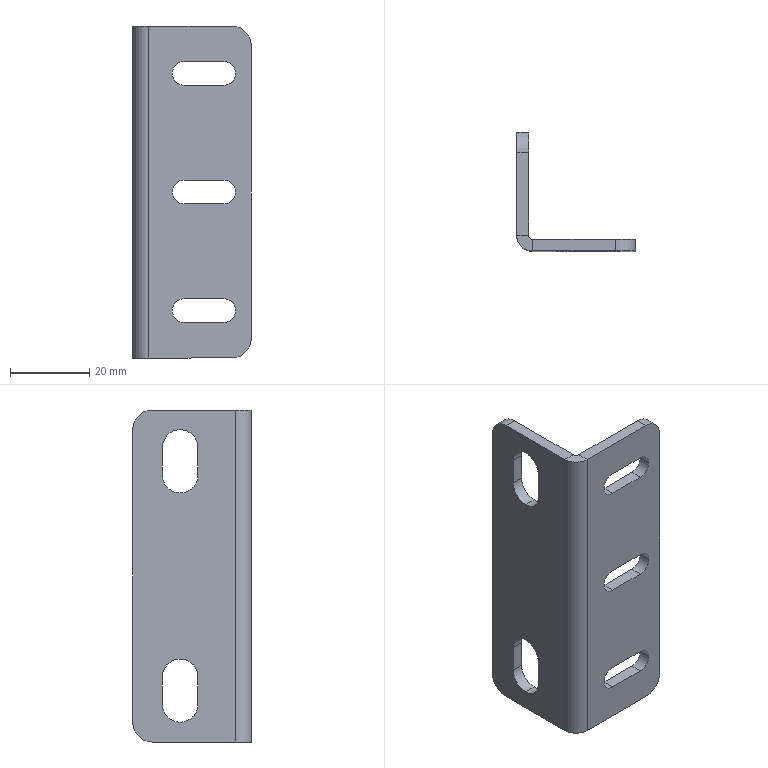Part | SolidWorks | features HoleWzd 2, EdgeFlange 1, Fillet 1, FlatPattern 1, SMBaseFlange 1, SheetMetal 1 | 1 solid | 40 faces | box 30 x 30 x 84 mm | volume 12475 mm3 | plane 22 | cylinder 18 | commonest cylinder face diameters 6 x6 9 x6 10 x4 2 x1 8 x1
STEP:
#1=CARTESIAN_POINT('',(-15.,15.,-37.));
#2=VERTEX_POINT('',#1);
#3=CARTESIAN_POINT('',(-15.,19.5,-32.5));
#4=VERTEX_POINT('',#3);
#5=CARTESIAN_POINT('',(-15.,15.,-32.5));
#6=DIRECTION('',(1.,0.,0.));
#7=DIRECTION('',(0.,0.,-1.));
#8=AXIS2_PLACEMENT_3D('',#5,#6,#7);
#9=CIRCLE('',#8,4.5);
#10=EDGE_CURVE('',#2,#4,#9,.T.);
#11=ORIENTED_EDGE('',*,*,#10,.F.);
#12=CARTESIAN_POINT('',(-12.,15.,-37.));
#13=VERTEX_POINT('',#12);
#14=CARTESIAN_POINT('',(-12.,15.,-37.));
#15=DIRECTION('',(1.,0.,0.));
#16=VECTOR('',#15,1000.);
#17=LINE('',#14,#16);
#18=EDGE_CURVE('',#2,#13,#17,.T.);
#19=ORIENTED_EDGE('',*,*,#18,.T.);
#20=CARTESIAN_POINT('',(-12.,19.5,-32.5));
#21=VERTEX_POINT('',#20);
#22=CARTESIAN_POINT('',(-12.,15.,-32.5));
#23=DIRECTION('',(1.,0.,0.));
#24=DIRECTION('',(0.,0.,-1.));
#25=AXIS2_PLACEMENT_3D('',#22,#23,#24);
#26=CIRCLE('',#25,4.5);
#27=EDGE_CURVE('',#13,#21,#26,.T.);
#28=ORIENTED_EDGE('',*,*,#27,.T.);
#29=CARTESIAN_POINT('',(-15.,19.5,-32.5));
#30=DIRECTION('',(-1.,0.,0.));
#31=VECTOR('',#30,1000.);
#32=LINE('',#29,#31);
#33=EDGE_CURVE('',#21,#4,#32,.T.);
#34=ORIENTED_EDGE('',*,*,#33,.T.);
#35=EDGE_LOOP('',(#11,#19,#28,#34));
#36=FACE_OUTER_BOUND('',#35,.T.);
#37=CARTESIAN_POINT('',(-12.,15.,-32.5));
#38=DIRECTION('',(1.,0.,0.));
#39=DIRECTION('',(0.,0.,-1.));
#40=AXIS2_PLACEMENT_3D('',#37,#38,#39);
#41=CYLINDRICAL_SURFACE('',#40,4.5);
#42=ADVANCED_FACE('',(#36),#41,.F.);
#43=CARTESIAN_POINT('',(-15.,15.,21.));
#44=VERTEX_POINT('',#43);
#45=CARTESIAN_POINT('',(-15.,19.5,25.5));
#46=VERTEX_POINT('',#45);
#47=CARTESIAN_POINT('',(-15.,15.,25.5));
#48=DIRECTION('',(1.,0.,0.));
#49=DIRECTION('',(0.,0.,-1.));
#50=AXIS2_PLACEMENT_3D('',#47,#48,#49);
#51=CIRCLE('',#50,4.5);
#52=EDGE_CURVE('',#44,#46,#51,.T.);
#53=ORIENTED_EDGE('',*,*,#52,.F.);
#54=CARTESIAN_POINT('',(-12.,15.,21.));
#55=VERTEX_POINT('',#54);
#56=CARTESIAN_POINT('',(-12.,15.,21.));
#57=DIRECTION('',(1.,0.,0.));
#58=VECTOR('',#57,1000.);
#59=LINE('',#56,#58);
#60=EDGE_CURVE('',#44,#55,#59,.T.);
#61=ORIENTED_EDGE('',*,*,#60,.T.);
#62=CARTESIAN_POINT('',(-12.,19.5,25.5));
#63=VERTEX_POINT('',#62);
#64=CARTESIAN_POINT('',(-12.,15.,25.5));
#65=DIRECTION('',(1.,0.,0.));
#66=DIRECTION('',(0.,0.,-1.));
#67=AXIS2_PLACEMENT_3D('',#64,#65,#66);
#68=CIRCLE('',#67,4.5);
#69=EDGE_CURVE('',#55,#63,#68,.T.);
#70=ORIENTED_EDGE('',*,*,#69,.T.);
#71=CARTESIAN_POINT('',(-15.,19.5,25.5));
#72=DIRECTION('',(-1.,0.,0.));
#73=VECTOR('',#72,1000.);
#74=LINE('',#71,#73);
#75=EDGE_CURVE('',#63,#46,#74,.T.);
#76=ORIENTED_EDGE('',*,*,#75,.T.);
#77=EDGE_LOOP('',(#53,#61,#70,#76));
#78=FACE_OUTER_BOUND('',#77,.T.);
#79=CARTESIAN_POINT('',(-12.,15.,25.5));
#80=DIRECTION('',(1.,0.,0.));
#81=DIRECTION('',(0.,0.,-1.));
#82=AXIS2_PLACEMENT_3D('',#79,#80,#81);
#83=CYLINDRICAL_SURFACE('',#82,4.5);
#84=ADVANCED_FACE('',(#78),#83,.F.);
#85=CARTESIAN_POINT('',(-15.,10.5,-32.5));
#86=VERTEX_POINT('',#85);
#87=CARTESIAN_POINT('',(-15.,15.,-32.5));
#88=DIRECTION('',(1.,0.,0.));
#89=DIRECTION('',(0.,0.,-1.));
#90=AXIS2_PLACEMENT_3D('',#87,#88,#89);
#91=CIRCLE('',#90,4.5);
#92=EDGE_CURVE('',#86,#2,#91,.T.);
#93=ORIENTED_EDGE('',*,*,#92,.T.);
#94=ORIENTED_EDGE('',*,*,#10,.T.);
#95=CARTESIAN_POINT('',(-15.,19.5,-25.5));
#96=VERTEX_POINT('',#95);
#97=CARTESIAN_POINT('',(-15.,19.5,-32.5));
#98=DIRECTION('',(0.,0.,1.));
#99=VECTOR('',#98,1000.);
#100=LINE('',#97,#99);
#101=EDGE_CURVE('',#4,#96,#100,.T.);
#102=ORIENTED_EDGE('',*,*,#101,.T.);
#103=CARTESIAN_POINT('',(-15.,10.5,-25.5));
#104=VERTEX_POINT('',#103);
#105=CARTESIAN_POINT('',(-15.,15.,-25.5));
#106=DIRECTION('',(1.,0.,0.));
#107=DIRECTION('',(0.,0.,-1.));
#108=AXIS2_PLACEMENT_3D('',#105,#106,#107);
#109=CIRCLE('',#108,4.5);
#110=EDGE_CURVE('',#96,#104,#109,.T.);
#111=ORIENTED_EDGE('',*,*,#110,.T.);
#112=CARTESIAN_POINT('',(-15.,10.5,-32.5));
#113=DIRECTION('',(0.,0.,1.));
#114=VECTOR('',#113,1000.);
#115=LINE('',#112,#114);
#116=EDGE_CURVE('',#86,#104,#115,.T.);
#117=ORIENTED_EDGE('',*,*,#116,.F.);
#118=EDGE_LOOP('',(#93,#94,#102,#111,#117));
#119=FACE_BOUND('',#118,.T.);
#120=CARTESIAN_POINT('',(-15.,27.,37.));
#121=VERTEX_POINT('',#120);
#122=CARTESIAN_POINT('',(-15.,27.,-37.));
#123=VERTEX_POINT('',#122);
#124=CARTESIAN_POINT('',(-15.,27.,0.));
#125=DIRECTION('',(0.,0.,-1.));
#126=VECTOR('',#125,1000.);
#127=LINE('',#124,#126);
#128=EDGE_CURVE('',#121,#123,#127,.T.);
#129=ORIENTED_EDGE('',*,*,#128,.T.);
#130=CARTESIAN_POINT('',(-15.,22.,-42.));
#131=VERTEX_POINT('',#130);
#132=CARTESIAN_POINT('',(-15.,22.,-37.));
#133=DIRECTION('',(-1.,0.,0.));
#134=DIRECTION('',(0.,1.,0.));
#135=AXIS2_PLACEMENT_3D('',#132,#133,#134);
#136=CIRCLE('',#135,5.);
#137=EDGE_CURVE('',#123,#131,#136,.T.);
#138=ORIENTED_EDGE('',*,*,#137,.T.);
#139=CARTESIAN_POINT('',(-15.,1.,-42.));
#140=VERTEX_POINT('',#139);
#141=CARTESIAN_POINT('',(-15.,0.,-42.));
#142=DIRECTION('',(0.,-1.,0.));
#143=VECTOR('',#142,1000.);
#144=LINE('',#141,#143);
#145=EDGE_CURVE('',#131,#140,#144,.T.);
#146=ORIENTED_EDGE('',*,*,#145,.T.);
#147=CARTESIAN_POINT('',(-15.,1.,42.));
#148=VERTEX_POINT('',#147);
#149=CARTESIAN_POINT('',(-15.,1.,-42.));
#150=DIRECTION('',(0.,0.,-1.));
#151=VECTOR('',#150,1000.);
#152=LINE('',#149,#151);
#153=EDGE_CURVE('',#148,#140,#152,.T.);
#154=ORIENTED_EDGE('',*,*,#153,.F.);
#155=CARTESIAN_POINT('',(-15.,22.,42.));
#156=VERTEX_POINT('',#155);
#157=CARTESIAN_POINT('',(-15.,0.,42.));
#158=DIRECTION('',(0.,1.,0.));
#159=VECTOR('',#158,1000.);
#160=LINE('',#157,#159);
#161=EDGE_CURVE('',#148,#156,#160,.T.);
#162=ORIENTED_EDGE('',*,*,#161,.T.);
#163=CARTESIAN_POINT('',(-15.,22.,37.));
#164=DIRECTION('',(-1.,0.,0.));
#165=DIRECTION('',(0.,1.,0.));
#166=AXIS2_PLACEMENT_3D('',#163,#164,#165);
#167=CIRCLE('',#166,5.);
#168=EDGE_CURVE('',#156,#121,#167,.T.);
#169=ORIENTED_EDGE('',*,*,#168,.T.);
#170=EDGE_LOOP('',(#129,#138,#146,#154,#162,#169));
#171=FACE_OUTER_BOUND('',#170,.T.);
#172=CARTESIAN_POINT('',(-15.,10.5,25.5));
#173=VERTEX_POINT('',#172);
#174=CARTESIAN_POINT('',(-15.,10.5,32.5));
#175=VERTEX_POINT('',#174);
#176=CARTESIAN_POINT('',(-15.,10.5,25.5));
#177=DIRECTION('',(0.,0.,1.));
#178=VECTOR('',#177,1000.);
#179=LINE('',#176,#178);
#180=EDGE_CURVE('',#173,#175,#179,.T.);
#181=ORIENTED_EDGE('',*,*,#180,.F.);
#182=CARTESIAN_POINT('',(-15.,15.,25.5));
#183=DIRECTION('',(1.,0.,0.));
#184=DIRECTION('',(0.,0.,-1.));
#185=AXIS2_PLACEMENT_3D('',#182,#183,#184);
#186=CIRCLE('',#185,4.5);
#187=EDGE_CURVE('',#173,#44,#186,.T.);
#188=ORIENTED_EDGE('',*,*,#187,.T.);
#189=ORIENTED_EDGE('',*,*,#52,.T.);
#190=CARTESIAN_POINT('',(-15.,19.5,32.5));
#191=VERTEX_POINT('',#190);
#192=CARTESIAN_POINT('',(-15.,19.5,25.5));
#193=DIRECTION('',(0.,0.,1.));
#194=VECTOR('',#193,1000.);
#195=LINE('',#192,#194);
#196=EDGE_CURVE('',#46,#191,#195,.T.);
#197=ORIENTED_EDGE('',*,*,#196,.T.);
#198=CARTESIAN_POINT('',(-15.,15.,32.5));
#199=DIRECTION('',(1.,0.,0.));
#200=DIRECTION('',(0.,0.,-1.));
#201=AXIS2_PLACEMENT_3D('',#198,#199,#200);
#202=CIRCLE('',#201,4.5);
#203=EDGE_CURVE('',#191,#175,#202,.T.);
#204=ORIENTED_EDGE('',*,*,#203,.T.);
#205=EDGE_LOOP('',(#181,#188,#189,#197,#204));
#206=FACE_BOUND('',#205,.T.);
#207=CARTESIAN_POINT('',(-15.,0.,0.));
#208=DIRECTION('',(1.,0.,0.));
#209=DIRECTION('',(0.,1.,0.));
#210=AXIS2_PLACEMENT_3D('',#207,#208,#209);
#211=PLANE('',#210);
#212=ADVANCED_FACE('',(#119,#171,#206),#211,.F.);
#213=CARTESIAN_POINT('',(-2.,0.,-33.));
#214=VERTEX_POINT('',#213);
#215=CARTESIAN_POINT('',(-2.,0.,-27.));
#216=VERTEX_POINT('',#215);
#217=CARTESIAN_POINT('',(-2.,0.,-30.));
#218=DIRECTION('',(0.,1.,0.));
#219=DIRECTION('',(0.,0.,1.));
#220=AXIS2_PLACEMENT_3D('',#217,#218,#219);
#221=CIRCLE('',#220,3.);
#222=EDGE_CURVE('',#214,#216,#221,.T.);
#223=ORIENTED_EDGE('',*,*,#222,.F.);
#224=CARTESIAN_POINT('',(8.,0.,-33.));
#225=VERTEX_POINT('',#224);
#226=CARTESIAN_POINT('',(-2.,0.,-33.));
#227=DIRECTION('',(1.,0.,0.));
#228=VECTOR('',#227,1000.);
#229=LINE('',#226,#228);
#230=EDGE_CURVE('',#214,#225,#229,.T.);
#231=ORIENTED_EDGE('',*,*,#230,.T.);
#232=CARTESIAN_POINT('',(8.,0.,-27.));
#233=VERTEX_POINT('',#232);
#234=CARTESIAN_POINT('',(8.,0.,-30.));
#235=DIRECTION('',(0.,1.,0.));
#236=DIRECTION('',(0.,0.,1.));
#237=AXIS2_PLACEMENT_3D('',#234,#235,#236);
#238=CIRCLE('',#237,3.);
#239=EDGE_CURVE('',#233,#225,#238,.T.);
#240=ORIENTED_EDGE('',*,*,#239,.F.);
#241=CARTESIAN_POINT('',(-2.,0.,-27.));
#242=DIRECTION('',(1.,0.,0.));
#243=VECTOR('',#242,1000.);
#244=LINE('',#241,#243);
#245=EDGE_CURVE('',#216,#233,#244,.T.);
#246=ORIENTED_EDGE('',*,*,#245,.F.);
#247=EDGE_LOOP('',(#223,#231,#240,#246));
#248=FACE_BOUND('',#247,.T.);
#249=CARTESIAN_POINT('',(-2.,0.,-3.));
#250=VERTEX_POINT('',#249);
#251=CARTESIAN_POINT('',(-2.,0.,3.));
#252=VERTEX_POINT('',#251);
#253=CARTESIAN_POINT('',(-2.,0.,0.));
#254=DIRECTION('',(0.,1.,0.));
#255=DIRECTION('',(0.,0.,1.));
#256=AXIS2_PLACEMENT_3D('',#253,#254,#255);
#257=CIRCLE('',#256,3.);
#258=EDGE_CURVE('',#250,#252,#257,.T.);
#259=ORIENTED_EDGE('',*,*,#258,.F.);
#260=CARTESIAN_POINT('',(8.,0.,-3.));
#261=VERTEX_POINT('',#260);
#262=CARTESIAN_POINT('',(-2.,0.,-3.));
#263=DIRECTION('',(1.,0.,0.));
#264=VECTOR('',#263,1000.);
#265=LINE('',#262,#264);
#266=EDGE_CURVE('',#250,#261,#265,.T.);
#267=ORIENTED_EDGE('',*,*,#266,.T.);
#268=CARTESIAN_POINT('',(8.,0.,3.));
#269=VERTEX_POINT('',#268);
#270=CARTESIAN_POINT('',(8.,0.,0.));
#271=DIRECTION('',(0.,1.,0.));
#272=DIRECTION('',(0.,0.,1.));
#273=AXIS2_PLACEMENT_3D('',#270,#271,#272);
#274=CIRCLE('',#273,3.);
#275=EDGE_CURVE('',#269,#261,#274,.T.);
#276=ORIENTED_EDGE('',*,*,#275,.F.);
#277=CARTESIAN_POINT('',(-2.,0.,3.));
#278=DIRECTION('',(1.,0.,0.));
#279=VECTOR('',#278,1000.);
#280=LINE('',#277,#279);
#281=EDGE_CURVE('',#252,#269,#280,.T.);
#282=ORIENTED_EDGE('',*,*,#281,.F.);
#283=EDGE_LOOP('',(#259,#267,#276,#282));
#284=FACE_BOUND('',#283,.T.);
#285=CARTESIAN_POINT('',(-2.,0.,27.));
#286=VERTEX_POINT('',#285);
#287=CARTESIAN_POINT('',(-2.,0.,33.));
#288=VERTEX_POINT('',#287);
#289=CARTESIAN_POINT('',(-2.,0.,30.));
#290=DIRECTION('',(0.,1.,0.));
#291=DIRECTION('',(0.,0.,1.));
#292=AXIS2_PLACEMENT_3D('',#289,#290,#291);
#293=CIRCLE('',#292,3.);
#294=EDGE_CURVE('',#286,#288,#293,.T.);
#295=ORIENTED_EDGE('',*,*,#294,.F.);
#296=CARTESIAN_POINT('',(8.,0.,27.));
#297=VERTEX_POINT('',#296);
#298=CARTESIAN_POINT('',(-2.,0.,27.));
#299=DIRECTION('',(1.,0.,0.));
#300=VECTOR('',#299,1000.);
#301=LINE('',#298,#300);
#302=EDGE_CURVE('',#286,#297,#301,.T.);
#303=ORIENTED_EDGE('',*,*,#302,.T.);
#304=CARTESIAN_POINT('',(8.,0.,33.));
#305=VERTEX_POINT('',#304);
#306=CARTESIAN_POINT('',(8.,0.,30.));
#307=DIRECTION('',(0.,1.,0.));
#308=DIRECTION('',(0.,0.,1.));
#309=AXIS2_PLACEMENT_3D('',#306,#307,#308);
#310=CIRCLE('',#309,3.);
#311=EDGE_CURVE('',#305,#297,#310,.T.);
#312=ORIENTED_EDGE('',*,*,#311,.F.);
#313=CARTESIAN_POINT('',(-2.,0.,33.));
#314=DIRECTION('',(1.,0.,0.));
#315=VECTOR('',#314,1000.);
#316=LINE('',#313,#315);
#317=EDGE_CURVE('',#288,#305,#316,.T.);
#318=ORIENTED_EDGE('',*,*,#317,.F.);
#319=EDGE_LOOP('',(#295,#303,#312,#318));
#320=FACE_BOUND('',#319,.T.);
#321=CARTESIAN_POINT('',(-11.,0.,42.));
#322=VERTEX_POINT('',#321);
#323=CARTESIAN_POINT('',(10.,0.,42.));
#324=VERTEX_POINT('',#323);
#325=CARTESIAN_POINT('',(15.,0.,42.));
#326=DIRECTION('',(1.,0.,0.));
#327=VECTOR('',#326,1000.);
#328=LINE('',#325,#327);
#329=EDGE_CURVE('',#322,#324,#328,.T.);
#330=ORIENTED_EDGE('',*,*,#329,.T.);
#331=CARTESIAN_POINT('',(15.,0.,37.));
#332=VERTEX_POINT('',#331);
#333=CARTESIAN_POINT('',(10.,0.,37.));
#334=DIRECTION('',(0.,1.,0.));
#335=DIRECTION('',(0.,0.,1.));
#336=AXIS2_PLACEMENT_3D('',#333,#334,#335);
#337=CIRCLE('',#336,5.);
#338=EDGE_CURVE('',#324,#332,#337,.T.);
#339=ORIENTED_EDGE('',*,*,#338,.T.);
#340=CARTESIAN_POINT('',(15.,0.,-37.));
#341=VERTEX_POINT('',#340);
#342=CARTESIAN_POINT('',(15.,0.,42.));
#343=DIRECTION('',(0.,0.,-1.));
#344=VECTOR('',#343,1000.);
#345=LINE('',#342,#344);
#346=EDGE_CURVE('',#332,#341,#345,.T.);
#347=ORIENTED_EDGE('',*,*,#346,.T.);
#348=CARTESIAN_POINT('',(10.,0.,-42.));
#349=VERTEX_POINT('',#348);
#350=CARTESIAN_POINT('',(10.,0.,-37.));
#351=DIRECTION('',(0.,1.,0.));
#352=DIRECTION('',(0.,0.,1.));
#353=AXIS2_PLACEMENT_3D('',#350,#351,#352);
#354=CIRCLE('',#353,5.);
#355=EDGE_CURVE('',#341,#349,#354,.T.);
#356=ORIENTED_EDGE('',*,*,#355,.T.);
#357=CARTESIAN_POINT('',(-11.,0.,-42.));
#358=VERTEX_POINT('',#357);
#359=CARTESIAN_POINT('',(15.,0.,-42.));
#360=DIRECTION('',(-1.,0.,0.));
#361=VECTOR('',#360,1000.);
#362=LINE('',#359,#361);
#363=EDGE_CURVE('',#349,#358,#362,.T.);
#364=ORIENTED_EDGE('',*,*,#363,.T.);
#365=CARTESIAN_POINT('',(-11.,0.,42.));
#366=DIRECTION('',(0.,0.,-1.));
#367=VECTOR('',#366,1000.);
#368=LINE('',#365,#367);
#369=EDGE_CURVE('',#322,#358,#368,.T.);
#370=ORIENTED_EDGE('',*,*,#369,.F.);
#371=EDGE_LOOP('',(#330,#339,#347,#356,#364,#370));
#372=FACE_OUTER_BOUND('',#371,.T.);
#373=CARTESIAN_POINT('',(0.,0.,0.));
#374=DIRECTION('',(0.,1.,0.));
#375=DIRECTION('',(0.,0.,1.));
#376=AXIS2_PLACEMENT_3D('',#373,#374,#375);
#377=PLANE('',#376);
#378=ADVANCED_FACE('',(#248,#284,#320,#372),#377,.T.);
#379=CARTESIAN_POINT('',(-2.,-3.,27.));
#380=VERTEX_POINT('',#379);
#381=CARTESIAN_POINT('',(8.,-3.,27.));
#382=VERTEX_POINT('',#381);
#383=CARTESIAN_POINT('',(-2.,-3.,27.));
#384=DIRECTION('',(1.,0.,0.));
#385=VECTOR('',#384,1000.);
#386=LINE('',#383,#385);
#387=EDGE_CURVE('',#380,#382,#386,.T.);
#388=ORIENTED_EDGE('',*,*,#387,.F.);
#389=CARTESIAN_POINT('',(-2.,-3.,33.));
#390=VERTEX_POINT('',#389);
#391=CARTESIAN_POINT('',(-2.,-3.,30.));
#392=DIRECTION('',(0.,1.,0.));
#393=DIRECTION('',(0.,0.,1.));
#394=AXIS2_PLACEMENT_3D('',#391,#392,#393);
#395=CIRCLE('',#394,3.);
#396=EDGE_CURVE('',#380,#390,#395,.T.);
#397=ORIENTED_EDGE('',*,*,#396,.T.);
#398=CARTESIAN_POINT('',(8.,-3.,33.));
#399=VERTEX_POINT('',#398);
#400=CARTESIAN_POINT('',(-2.,-3.,33.));
#401=DIRECTION('',(1.,0.,0.));
#402=VECTOR('',#401,1000.);
#403=LINE('',#400,#402);
#404=EDGE_CURVE('',#390,#399,#403,.T.);
#405=ORIENTED_EDGE('',*,*,#404,.T.);
#406=CARTESIAN_POINT('',(8.,-3.,30.));
#407=DIRECTION('',(0.,1.,0.));
#408=DIRECTION('',(0.,0.,1.));
#409=AXIS2_PLACEMENT_3D('',#406,#407,#408);
#410=CIRCLE('',#409,3.);
#411=EDGE_CURVE('',#399,#382,#410,.T.);
#412=ORIENTED_EDGE('',*,*,#411,.T.);
#413=EDGE_LOOP('',(#388,#397,#405,#412));
#414=FACE_BOUND('',#413,.T.);
#415=CARTESIAN_POINT('',(-2.,-3.,3.));
#416=VERTEX_POINT('',#415);
#417=CARTESIAN_POINT('',(8.,-3.,3.));
#418=VERTEX_POINT('',#417);
#419=CARTESIAN_POINT('',(-2.,-3.,3.));
#420=DIRECTION('',(1.,0.,0.));
#421=VECTOR('',#420,1000.);
#422=LINE('',#419,#421);
#423=EDGE_CURVE('',#416,#418,#422,.T.);
#424=ORIENTED_EDGE('',*,*,#423,.T.);
#425=CARTESIAN_POINT('',(8.,-3.,-3.));
#426=VERTEX_POINT('',#425);
#427=CARTESIAN_POINT('',(8.,-3.,0.));
#428=DIRECTION('',(0.,1.,0.));
#429=DIRECTION('',(0.,0.,1.));
#430=AXIS2_PLACEMENT_3D('',#427,#428,#429);
#431=CIRCLE('',#430,3.);
#432=EDGE_CURVE('',#418,#426,#431,.T.);
#433=ORIENTED_EDGE('',*,*,#432,.T.);
#434=CARTESIAN_POINT('',(-2.,-3.,-3.));
#435=VERTEX_POINT('',#434);
#436=CARTESIAN_POINT('',(-2.,-3.,-3.));
#437=DIRECTION('',(1.,0.,0.));
#438=VECTOR('',#437,1000.);
#439=LINE('',#436,#438);
#440=EDGE_CURVE('',#435,#426,#439,.T.);
#441=ORIENTED_EDGE('',*,*,#440,.F.);
#442=CARTESIAN_POINT('',(-2.,-3.,0.));
#443=DIRECTION('',(0.,1.,0.));
#444=DIRECTION('',(0.,0.,1.));
#445=AXIS2_PLACEMENT_3D('',#442,#443,#444);
#446=CIRCLE('',#445,3.);
#447=EDGE_CURVE('',#435,#416,#446,.T.);
#448=ORIENTED_EDGE('',*,*,#447,.T.);
#449=EDGE_LOOP('',(#424,#433,#441,#448));
#450=FACE_BOUND('',#449,.T.);
#451=CARTESIAN_POINT('',(-2.,-3.,-33.));
#452=VERTEX_POINT('',#451);
#453=CARTESIAN_POINT('',(-2.,-3.,-27.));
#454=VERTEX_POINT('',#453);
#455=CARTESIAN_POINT('',(-2.,-3.,-30.));
#456=DIRECTION('',(0.,1.,0.));
#457=DIRECTION('',(0.,0.,1.));
#458=AXIS2_PLACEMENT_3D('',#455,#456,#457);
#459=CIRCLE('',#458,3.);
#460=EDGE_CURVE('',#452,#454,#459,.T.);
#461=ORIENTED_EDGE('',*,*,#460,.T.);
#462=CARTESIAN_POINT('',(8.,-3.,-27.));
#463=VERTEX_POINT('',#462);
#464=CARTESIAN_POINT('',(-2.,-3.,-27.));
#465=DIRECTION('',(1.,0.,0.));
#466=VECTOR('',#465,1000.);
#467=LINE('',#464,#466);
#468=EDGE_CURVE('',#454,#463,#467,.T.);
#469=ORIENTED_EDGE('',*,*,#468,.T.);
#470=CARTESIAN_POINT('',(8.,-3.,-33.));
#471=VERTEX_POINT('',#470);
#472=CARTESIAN_POINT('',(8.,-3.,-30.));
#473=DIRECTION('',(0.,1.,0.));
#474=DIRECTION('',(0.,0.,1.));
#475=AXIS2_PLACEMENT_3D('',#472,#473,#474);
#476=CIRCLE('',#475,3.);
#477=EDGE_CURVE('',#463,#471,#476,.T.);
#478=ORIENTED_EDGE('',*,*,#477,.T.);
#479=CARTESIAN_POINT('',(-2.,-3.,-33.));
#480=DIRECTION('',(1.,0.,0.));
#481=VECTOR('',#480,1000.);
#482=LINE('',#479,#481);
#483=EDGE_CURVE('',#452,#471,#482,.T.);
#484=ORIENTED_EDGE('',*,*,#483,.F.);
#485=EDGE_LOOP('',(#461,#469,#478,#484));
#486=FACE_BOUND('',#485,.T.);
#487=CARTESIAN_POINT('',(15.,-3.,37.));
#488=VERTEX_POINT('',#487);
#489=CARTESIAN_POINT('',(15.,-3.,-37.));
#490=VERTEX_POINT('',#489);
#491=CARTESIAN_POINT('',(15.,-3.,42.));
#492=DIRECTION('',(0.,0.,-1.));
#493=VECTOR('',#492,1000.);
#494=LINE('',#491,#493);
#495=EDGE_CURVE('',#488,#490,#494,.T.);
#496=ORIENTED_EDGE('',*,*,#495,.F.);
#497=CARTESIAN_POINT('',(10.,-3.,42.));
#498=VERTEX_POINT('',#497);
#499=CARTESIAN_POINT('',(10.,-3.,37.));
#500=DIRECTION('',(0.,-1.,0.));
#501=DIRECTION('',(0.,0.,1.));
#502=AXIS2_PLACEMENT_3D('',#499,#500,#501);
#503=CIRCLE('',#502,5.);
#504=EDGE_CURVE('',#488,#498,#503,.T.);
#505=ORIENTED_EDGE('',*,*,#504,.T.);
#506=CARTESIAN_POINT('',(-11.,-3.,42.));
#507=VERTEX_POINT('',#506);
#508=CARTESIAN_POINT('',(15.,-3.,42.));
#509=DIRECTION('',(1.,0.,0.));
#510=VECTOR('',#509,1000.);
#511=LINE('',#508,#510);
#512=EDGE_CURVE('',#507,#498,#511,.T.);
#513=ORIENTED_EDGE('',*,*,#512,.F.);
#514=CARTESIAN_POINT('',(-11.,-3.,-42.));
#515=VERTEX_POINT('',#514);
#516=CARTESIAN_POINT('',(-11.,-3.,42.));
#517=DIRECTION('',(0.,0.,-1.));
#518=VECTOR('',#517,1000.);
#519=LINE('',#516,#518);
#520=EDGE_CURVE('',#507,#515,#519,.T.);
#521=ORIENTED_EDGE('',*,*,#520,.T.);
#522=CARTESIAN_POINT('',(10.,-3.,-42.));
#523=VERTEX_POINT('',#522);
#524=CARTESIAN_POINT('',(15.,-3.,-42.));
#525=DIRECTION('',(-1.,0.,0.));
#526=VECTOR('',#525,1000.);
#527=LINE('',#524,#526);
#528=EDGE_CURVE('',#523,#515,#527,.T.);
#529=ORIENTED_EDGE('',*,*,#528,.F.);
#530=CARTESIAN_POINT('',(10.,-3.,-37.));
#531=DIRECTION('',(0.,-1.,0.));
#532=DIRECTION('',(0.,0.,1.));
#533=AXIS2_PLACEMENT_3D('',#530,#531,#532);
#534=CIRCLE('',#533,5.);
#535=EDGE_CURVE('',#523,#490,#534,.T.);
#536=ORIENTED_EDGE('',*,*,#535,.T.);
#537=EDGE_LOOP('',(#496,#505,#513,#521,#529,#536));
#538=FACE_OUTER_BOUND('',#537,.T.);
#539=CARTESIAN_POINT('',(0.,-3.,0.));
#540=DIRECTION('',(0.,1.,0.));
#541=DIRECTION('',(0.,0.,1.));
#542=AXIS2_PLACEMENT_3D('',#539,#540,#541);
#543=PLANE('',#542);
#544=ADVANCED_FACE('',(#414,#450,#486,#538),#543,.F.);
#545=ORIENTED_EDGE('',*,*,#512,.T.);
#546=CARTESIAN_POINT('',(10.,-3.,42.));
#547=DIRECTION('',(0.,1.,0.));
#548=VECTOR('',#547,1000.);
#549=LINE('',#546,#548);
#550=EDGE_CURVE('',#498,#324,#549,.T.);
#551=ORIENTED_EDGE('',*,*,#550,.T.);
#552=ORIENTED_EDGE('',*,*,#329,.F.);
#553=CARTESIAN_POINT('',(-11.,0.,42.));
#554=DIRECTION('',(0.,-1.,0.));
#555=VECTOR('',#554,1000.);
#556=LINE('',#553,#555);
#557=EDGE_CURVE('',#322,#507,#556,.T.);
#558=ORIENTED_EDGE('',*,*,#557,.T.);
#559=EDGE_LOOP('',(#545,#551,#552,#558));
#560=FACE_OUTER_BOUND('',#559,.T.);
#561=CARTESIAN_POINT('',(15.,-3.,42.));
#562=DIRECTION('',(0.,0.,1.));
#563=DIRECTION('',(1.,0.,0.));
#564=AXIS2_PLACEMENT_3D('',#561,#562,#563);
#565=PLANE('',#564);
#566=ADVANCED_FACE('',(#560),#565,.T.);
#567=ORIENTED_EDGE('',*,*,#363,.F.);
#568=CARTESIAN_POINT('',(10.,-3.,-42.));
#569=DIRECTION('',(0.,-1.,0.));
#570=VECTOR('',#569,1000.);
#571=LINE('',#568,#570);
#572=EDGE_CURVE('',#349,#523,#571,.T.);
#573=ORIENTED_EDGE('',*,*,#572,.T.);
#574=ORIENTED_EDGE('',*,*,#528,.T.);
#575=CARTESIAN_POINT('',(-11.,0.,-42.));
#576=DIRECTION('',(0.,-1.,0.));
#577=VECTOR('',#576,1000.);
#578=LINE('',#575,#577);
#579=EDGE_CURVE('',#358,#515,#578,.T.);
#580=ORIENTED_EDGE('',*,*,#579,.F.);
#581=EDGE_LOOP('',(#567,#573,#574,#580));
#582=FACE_OUTER_BOUND('',#581,.T.);
#583=CARTESIAN_POINT('',(15.,-3.,-42.));
#584=DIRECTION('',(0.,0.,-1.));
#585=DIRECTION('',(-1.,0.,0.));
#586=AXIS2_PLACEMENT_3D('',#583,#584,#585);
#587=PLANE('',#586);
#588=ADVANCED_FACE('',(#582),#587,.T.);
#589=ORIENTED_EDGE('',*,*,#346,.F.);
#590=CARTESIAN_POINT('',(15.,-3.,37.));
#591=DIRECTION('',(0.,-1.,0.));
#592=VECTOR('',#591,1000.);
#593=LINE('',#590,#592);
#594=EDGE_CURVE('',#332,#488,#593,.T.);
#595=ORIENTED_EDGE('',*,*,#594,.T.);
#596=ORIENTED_EDGE('',*,*,#495,.T.);
#597=CARTESIAN_POINT('',(15.,-3.,-37.));
#598=DIRECTION('',(0.,1.,0.));
#599=VECTOR('',#598,1000.);
#600=LINE('',#597,#599);
#601=EDGE_CURVE('',#490,#341,#600,.T.);
#602=ORIENTED_EDGE('',*,*,#601,.T.);
#603=EDGE_LOOP('',(#589,#595,#596,#602));
#604=FACE_OUTER_BOUND('',#603,.T.);
#605=CARTESIAN_POINT('',(15.,-3.,42.));
#606=DIRECTION('',(1.,0.,0.));
#607=DIRECTION('',(0.,0.,-1.));
#608=AXIS2_PLACEMENT_3D('',#605,#606,#607);
#609=PLANE('',#608);
#610=ADVANCED_FACE('',(#604),#609,.T.);
#611=ORIENTED_EDGE('',*,*,#411,.F.);
#612=CARTESIAN_POINT('',(8.,0.,33.));
#613=DIRECTION('',(0.,-1.,0.));
#614=VECTOR('',#613,1000.);
#615=LINE('',#612,#614);
#616=EDGE_CURVE('',#305,#399,#615,.T.);
#617=ORIENTED_EDGE('',*,*,#616,.F.);
#618=ORIENTED_EDGE('',*,*,#311,.T.);
#619=CARTESIAN_POINT('',(8.,0.,27.));
#620=DIRECTION('',(0.,1.,0.));
#621=VECTOR('',#620,1000.);
#622=LINE('',#619,#621);
#623=EDGE_CURVE('',#382,#297,#622,.T.);
#624=ORIENTED_EDGE('',*,*,#623,.F.);
#625=EDGE_LOOP('',(#611,#617,#618,#624));
#626=FACE_OUTER_BOUND('',#625,.T.);
#627=CARTESIAN_POINT('',(8.,0.,30.));
#628=DIRECTION('',(0.,1.,0.));
#629=DIRECTION('',(0.,0.,1.));
#630=AXIS2_PLACEMENT_3D('',#627,#628,#629);
#631=CYLINDRICAL_SURFACE('',#630,3.);
#632=ADVANCED_FACE('',(#626),#631,.F.);
#633=ORIENTED_EDGE('',*,*,#294,.T.);
#634=CARTESIAN_POINT('',(-2.,0.,33.));
#635=DIRECTION('',(0.,1.,0.));
#636=VECTOR('',#635,1000.);
#637=LINE('',#634,#636);
#638=EDGE_CURVE('',#390,#288,#637,.T.);
#639=ORIENTED_EDGE('',*,*,#638,.F.);
#640=ORIENTED_EDGE('',*,*,#396,.F.);
#641=CARTESIAN_POINT('',(-2.,0.,27.));
#642=DIRECTION('',(0.,-1.,0.));
#643=VECTOR('',#642,1000.);
#644=LINE('',#641,#643);
#645=EDGE_CURVE('',#286,#380,#644,.T.);
#646=ORIENTED_EDGE('',*,*,#645,.F.);
#647=EDGE_LOOP('',(#633,#639,#640,#646));
#648=FACE_OUTER_BOUND('',#647,.T.);
#649=CARTESIAN_POINT('',(-2.,0.,30.));
#650=DIRECTION('',(0.,1.,0.));
#651=DIRECTION('',(0.,0.,1.));
#652=AXIS2_PLACEMENT_3D('',#649,#650,#651);
#653=CYLINDRICAL_SURFACE('',#652,3.);
#654=ADVANCED_FACE('',(#648),#653,.F.);
#655=ORIENTED_EDGE('',*,*,#623,.T.);
#656=ORIENTED_EDGE('',*,*,#302,.F.);
#657=ORIENTED_EDGE('',*,*,#645,.T.);
#658=ORIENTED_EDGE('',*,*,#387,.T.);
#659=EDGE_LOOP('',(#655,#656,#657,#658));
#660=FACE_OUTER_BOUND('',#659,.T.);
#661=CARTESIAN_POINT('',(-2.,0.,27.));
#662=DIRECTION('',(0.,0.,-1.));
#663=DIRECTION('',(-1.,0.,0.));
#664=AXIS2_PLACEMENT_3D('',#661,#662,#663);
#665=PLANE('',#664);
#666=ADVANCED_FACE('',(#660),#665,.F.);
#667=ORIENTED_EDGE('',*,*,#616,.T.);
#668=ORIENTED_EDGE('',*,*,#404,.F.);
#669=ORIENTED_EDGE('',*,*,#638,.T.);
#670=ORIENTED_EDGE('',*,*,#317,.T.);
#671=EDGE_LOOP('',(#667,#668,#669,#670));
#672=FACE_OUTER_BOUND('',#671,.T.);
#673=CARTESIAN_POINT('',(-2.,0.,33.));
#674=DIRECTION('',(0.,0.,1.));
#675=DIRECTION('',(1.,0.,0.));
#676=AXIS2_PLACEMENT_3D('',#673,#674,#675);
#677=PLANE('',#676);
#678=ADVANCED_FACE('',(#672),#677,.F.);
#679=ORIENTED_EDGE('',*,*,#432,.F.);
#680=CARTESIAN_POINT('',(8.,0.,3.));
#681=DIRECTION('',(0.,-1.,0.));
#682=VECTOR('',#681,1000.);
#683=LINE('',#680,#682);
#684=EDGE_CURVE('',#269,#418,#683,.T.);
#685=ORIENTED_EDGE('',*,*,#684,.F.);
#686=ORIENTED_EDGE('',*,*,#275,.T.);
#687=CARTESIAN_POINT('',(8.,0.,-3.));
#688=DIRECTION('',(0.,1.,0.));
#689=VECTOR('',#688,1000.);
#690=LINE('',#687,#689);
#691=EDGE_CURVE('',#426,#261,#690,.T.);
#692=ORIENTED_EDGE('',*,*,#691,.F.);
#693=EDGE_LOOP('',(#679,#685,#686,#692));
#694=FACE_OUTER_BOUND('',#693,.T.);
#695=CARTESIAN_POINT('',(8.,0.,0.));
#696=DIRECTION('',(0.,1.,0.));
#697=DIRECTION('',(0.,0.,1.));
#698=AXIS2_PLACEMENT_3D('',#695,#696,#697);
#699=CYLINDRICAL_SURFACE('',#698,3.);
#700=ADVANCED_FACE('',(#694),#699,.F.);
#701=ORIENTED_EDGE('',*,*,#258,.T.);
#702=CARTESIAN_POINT('',(-2.,0.,3.));
#703=DIRECTION('',(0.,1.,0.));
#704=VECTOR('',#703,1000.);
#705=LINE('',#702,#704);
#706=EDGE_CURVE('',#416,#252,#705,.T.);
#707=ORIENTED_EDGE('',*,*,#706,.F.);
#708=ORIENTED_EDGE('',*,*,#447,.F.);
#709=CARTESIAN_POINT('',(-2.,0.,-3.));
#710=DIRECTION('',(0.,-1.,0.));
#711=VECTOR('',#710,1000.);
#712=LINE('',#709,#711);
#713=EDGE_CURVE('',#250,#435,#712,.T.);
#714=ORIENTED_EDGE('',*,*,#713,.F.);
#715=EDGE_LOOP('',(#701,#707,#708,#714));
#716=FACE_OUTER_BOUND('',#715,.T.);
#717=CARTESIAN_POINT('',(-2.,0.,0.));
#718=DIRECTION('',(0.,1.,0.));
#719=DIRECTION('',(0.,0.,1.));
#720=AXIS2_PLACEMENT_3D('',#717,#718,#719);
#721=CYLINDRICAL_SURFACE('',#720,3.);
#722=ADVANCED_FACE('',(#716),#721,.F.);
#723=ORIENTED_EDGE('',*,*,#691,.T.);
#724=ORIENTED_EDGE('',*,*,#266,.F.);
#725=ORIENTED_EDGE('',*,*,#713,.T.);
#726=ORIENTED_EDGE('',*,*,#440,.T.);
#727=EDGE_LOOP('',(#723,#724,#725,#726));
#728=FACE_OUTER_BOUND('',#727,.T.);
#729=CARTESIAN_POINT('',(-2.,0.,-3.));
#730=DIRECTION('',(0.,0.,-1.));
#731=DIRECTION('',(-1.,0.,0.));
#732=AXIS2_PLACEMENT_3D('',#729,#730,#731);
#733=PLANE('',#732);
#734=ADVANCED_FACE('',(#728),#733,.F.);
#735=ORIENTED_EDGE('',*,*,#684,.T.);
#736=ORIENTED_EDGE('',*,*,#423,.F.);
#737=ORIENTED_EDGE('',*,*,#706,.T.);
#738=ORIENTED_EDGE('',*,*,#281,.T.);
#739=EDGE_LOOP('',(#735,#736,#737,#738));
#740=FACE_OUTER_BOUND('',#739,.T.);
#741=CARTESIAN_POINT('',(-2.,0.,3.));
#742=DIRECTION('',(0.,0.,1.));
#743=DIRECTION('',(1.,0.,0.));
#744=AXIS2_PLACEMENT_3D('',#741,#742,#743);
#745=PLANE('',#744);
#746=ADVANCED_FACE('',(#740),#745,.F.);
#747=ORIENTED_EDGE('',*,*,#477,.F.);
#748=CARTESIAN_POINT('',(8.,0.,-27.));
#749=DIRECTION('',(0.,-1.,0.));
#750=VECTOR('',#749,1000.);
#751=LINE('',#748,#750);
#752=EDGE_CURVE('',#233,#463,#751,.T.);
#753=ORIENTED_EDGE('',*,*,#752,.F.);
#754=ORIENTED_EDGE('',*,*,#239,.T.);
#755=CARTESIAN_POINT('',(8.,0.,-33.));
#756=DIRECTION('',(0.,1.,0.));
#757=VECTOR('',#756,1000.);
#758=LINE('',#755,#757);
#759=EDGE_CURVE('',#471,#225,#758,.T.);
#760=ORIENTED_EDGE('',*,*,#759,.F.);
#761=EDGE_LOOP('',(#747,#753,#754,#760));
#762=FACE_OUTER_BOUND('',#761,.T.);
#763=CARTESIAN_POINT('',(8.,0.,-30.));
#764=DIRECTION('',(0.,1.,0.));
#765=DIRECTION('',(0.,0.,1.));
#766=AXIS2_PLACEMENT_3D('',#763,#764,#765);
#767=CYLINDRICAL_SURFACE('',#766,3.);
#768=ADVANCED_FACE('',(#762),#767,.F.);
#769=ORIENTED_EDGE('',*,*,#222,.T.);
#770=CARTESIAN_POINT('',(-2.,0.,-27.));
#771=DIRECTION('',(0.,1.,0.));
#772=VECTOR('',#771,1000.);
#773=LINE('',#770,#772);
#774=EDGE_CURVE('',#454,#216,#773,.T.);
#775=ORIENTED_EDGE('',*,*,#774,.F.);
#776=ORIENTED_EDGE('',*,*,#460,.F.);
#777=CARTESIAN_POINT('',(-2.,0.,-33.));
#778=DIRECTION('',(0.,-1.,0.));
#779=VECTOR('',#778,1000.);
#780=LINE('',#777,#779);
#781=EDGE_CURVE('',#214,#452,#780,.T.);
#782=ORIENTED_EDGE('',*,*,#781,.F.);
#783=EDGE_LOOP('',(#769,#775,#776,#782));
#784=FACE_OUTER_BOUND('',#783,.T.);
#785=CARTESIAN_POINT('',(-2.,0.,-30.));
#786=DIRECTION('',(0.,1.,0.));
#787=DIRECTION('',(0.,0.,1.));
#788=AXIS2_PLACEMENT_3D('',#785,#786,#787);
#789=CYLINDRICAL_SURFACE('',#788,3.);
#790=ADVANCED_FACE('',(#784),#789,.F.);
#791=ORIENTED_EDGE('',*,*,#759,.T.);
#792=ORIENTED_EDGE('',*,*,#230,.F.);
#793=ORIENTED_EDGE('',*,*,#781,.T.);
#794=ORIENTED_EDGE('',*,*,#483,.T.);
#795=EDGE_LOOP('',(#791,#792,#793,#794));
#796=FACE_OUTER_BOUND('',#795,.T.);
#797=CARTESIAN_POINT('',(-2.,0.,-33.));
#798=DIRECTION('',(0.,0.,-1.));
#799=DIRECTION('',(-1.,0.,0.));
#800=AXIS2_PLACEMENT_3D('',#797,#798,#799);
#801=PLANE('',#800);
#802=ADVANCED_FACE('',(#796),#801,.F.);
#803=ORIENTED_EDGE('',*,*,#752,.T.);
#804=ORIENTED_EDGE('',*,*,#468,.F.);
#805=ORIENTED_EDGE('',*,*,#774,.T.);
#806=ORIENTED_EDGE('',*,*,#245,.T.);
#807=EDGE_LOOP('',(#803,#804,#805,#806));
#808=FACE_OUTER_BOUND('',#807,.T.);
#809=CARTESIAN_POINT('',(-2.,0.,-27.));
#810=DIRECTION('',(0.,0.,1.));
#811=DIRECTION('',(1.,0.,0.));
#812=AXIS2_PLACEMENT_3D('',#809,#810,#811);
#813=PLANE('',#812);
#814=ADVANCED_FACE('',(#808),#813,.F.);
#815=CARTESIAN_POINT('',(-12.,1.,-42.));
#816=VERTEX_POINT('',#815);
#817=CARTESIAN_POINT('',(-15.,1.,-42.));
#818=DIRECTION('',(-1.,0.,0.));
#819=VECTOR('',#818,1000.);
#820=LINE('',#817,#819);
#821=EDGE_CURVE('',#816,#140,#820,.T.);
#822=ORIENTED_EDGE('',*,*,#821,.F.);
#823=CARTESIAN_POINT('',(-11.,1.,-42.));
#824=DIRECTION('',(0.,0.,-1.));
#825=DIRECTION('',(1.,0.,0.));
#826=AXIS2_PLACEMENT_3D('',#823,#824,#825);
#827=CIRCLE('',#826,1.);
#828=EDGE_CURVE('',#358,#816,#827,.T.);
#829=ORIENTED_EDGE('',*,*,#828,.F.);
#830=ORIENTED_EDGE('',*,*,#579,.T.);
#831=CARTESIAN_POINT('',(-11.,1.,-42.));
#832=DIRECTION('',(0.,0.,-1.));
#833=DIRECTION('',(1.,0.,0.));
#834=AXIS2_PLACEMENT_3D('',#831,#832,#833);
#835=CIRCLE('',#834,4.);
#836=EDGE_CURVE('',#515,#140,#835,.T.);
#837=ORIENTED_EDGE('',*,*,#836,.T.);
#838=EDGE_LOOP('',(#822,#829,#830,#837));
#839=FACE_OUTER_BOUND('',#838,.T.);
#840=CARTESIAN_POINT('',(-11.,1.,-42.));
#841=DIRECTION('',(0.,0.,-1.));
#842=DIRECTION('',(-1.,0.,0.));
#843=AXIS2_PLACEMENT_3D('',#840,#841,#842);
#844=PLANE('',#843);
#845=ADVANCED_FACE('',(#839),#844,.T.);
#846=CARTESIAN_POINT('',(-12.,1.,42.));
#847=VERTEX_POINT('',#846);
#848=CARTESIAN_POINT('',(-11.,1.,42.));
#849=DIRECTION('',(0.,0.,1.));
#850=DIRECTION('',(1.,0.,0.));
#851=AXIS2_PLACEMENT_3D('',#848,#849,#850);
#852=CIRCLE('',#851,1.);
#853=EDGE_CURVE('',#847,#322,#852,.T.);
#854=ORIENTED_EDGE('',*,*,#853,.F.);
#855=CARTESIAN_POINT('',(-12.,1.,42.));
#856=DIRECTION('',(-1.,0.,0.));
#857=VECTOR('',#856,1000.);
#858=LINE('',#855,#857);
#859=EDGE_CURVE('',#847,#148,#858,.T.);
#860=ORIENTED_EDGE('',*,*,#859,.T.);
#861=CARTESIAN_POINT('',(-11.,1.,42.));
#862=DIRECTION('',(0.,0.,1.));
#863=DIRECTION('',(1.,0.,0.));
#864=AXIS2_PLACEMENT_3D('',#861,#862,#863);
#865=CIRCLE('',#864,4.);
#866=EDGE_CURVE('',#148,#507,#865,.T.);
#867=ORIENTED_EDGE('',*,*,#866,.T.);
#868=ORIENTED_EDGE('',*,*,#557,.F.);
#869=EDGE_LOOP('',(#854,#860,#867,#868));
#870=FACE_OUTER_BOUND('',#869,.T.);
#871=CARTESIAN_POINT('',(-11.,1.,42.));
#872=DIRECTION('',(0.,0.,-1.));
#873=DIRECTION('',(-1.,0.,0.));
#874=AXIS2_PLACEMENT_3D('',#871,#872,#873);
#875=PLANE('',#874);
#876=ADVANCED_FACE('',(#870),#875,.F.);
#877=ORIENTED_EDGE('',*,*,#520,.F.);
#878=ORIENTED_EDGE('',*,*,#866,.F.);
#879=ORIENTED_EDGE('',*,*,#153,.T.);
#880=ORIENTED_EDGE('',*,*,#836,.F.);
#881=EDGE_LOOP('',(#877,#878,#879,#880));
#882=FACE_OUTER_BOUND('',#881,.T.);
#883=CARTESIAN_POINT('',(-11.,1.,42.));
#884=DIRECTION('',(0.,0.,1.));
#885=DIRECTION('',(-1.,0.,0.));
#886=AXIS2_PLACEMENT_3D('',#883,#884,#885);
#887=CYLINDRICAL_SURFACE('',#886,4.);
#888=ADVANCED_FACE('',(#882),#887,.T.);
#889=ORIENTED_EDGE('',*,*,#369,.T.);
#890=ORIENTED_EDGE('',*,*,#828,.T.);
#891=CARTESIAN_POINT('',(-12.,1.,-42.));
#892=DIRECTION('',(0.,0.,1.));
#893=VECTOR('',#892,1000.);
#894=LINE('',#891,#893);
#895=EDGE_CURVE('',#816,#847,#894,.T.);
#896=ORIENTED_EDGE('',*,*,#895,.T.);
#897=ORIENTED_EDGE('',*,*,#853,.T.);
#898=EDGE_LOOP('',(#889,#890,#896,#897));
#899=FACE_OUTER_BOUND('',#898,.T.);
#900=CARTESIAN_POINT('',(-11.,1.,42.));
#901=DIRECTION('',(0.,0.,1.));
#902=DIRECTION('',(-1.,0.,0.));
#903=AXIS2_PLACEMENT_3D('',#900,#901,#902);
#904=CYLINDRICAL_SURFACE('',#903,1.);
#905=ADVANCED_FACE('',(#899),#904,.F.);
#906=ORIENTED_EDGE('',*,*,#145,.F.);
#907=CARTESIAN_POINT('',(-12.,22.,-42.));
#908=VERTEX_POINT('',#907);
#909=CARTESIAN_POINT('',(-15.,22.,-42.));
#910=DIRECTION('',(1.,0.,0.));
#911=VECTOR('',#910,1000.);
#912=LINE('',#909,#911);
#913=EDGE_CURVE('',#131,#908,#912,.T.);
#914=ORIENTED_EDGE('',*,*,#913,.T.);
#915=CARTESIAN_POINT('',(-12.,0.,-42.));
#916=DIRECTION('',(0.,-1.,0.));
#917=VECTOR('',#916,1000.);
#918=LINE('',#915,#917);
#919=EDGE_CURVE('',#908,#816,#918,.T.);
#920=ORIENTED_EDGE('',*,*,#919,.T.);
#921=ORIENTED_EDGE('',*,*,#821,.T.);
#922=EDGE_LOOP('',(#906,#914,#920,#921));
#923=FACE_OUTER_BOUND('',#922,.T.);
#924=CARTESIAN_POINT('',(-15.,0.,-42.));
#925=DIRECTION('',(0.,0.,1.));
#926=DIRECTION('',(1.,0.,0.));
#927=AXIS2_PLACEMENT_3D('',#924,#925,#926);
#928=PLANE('',#927);
#929=ADVANCED_FACE('',(#923),#928,.F.);
#930=CARTESIAN_POINT('',(-12.,22.,42.));
#931=VERTEX_POINT('',#930);
#932=CARTESIAN_POINT('',(-12.,27.,42.));
#933=DIRECTION('',(0.,1.,0.));
#934=VECTOR('',#933,1000.);
#935=LINE('',#932,#934);
#936=EDGE_CURVE('',#847,#931,#935,.T.);
#937=ORIENTED_EDGE('',*,*,#936,.T.);
#938=CARTESIAN_POINT('',(-15.,22.,42.));
#939=DIRECTION('',(-1.,0.,0.));
#940=VECTOR('',#939,1000.);
#941=LINE('',#938,#940);
#942=EDGE_CURVE('',#931,#156,#941,.T.);
#943=ORIENTED_EDGE('',*,*,#942,.T.);
#944=ORIENTED_EDGE('',*,*,#161,.F.);
#945=ORIENTED_EDGE('',*,*,#859,.F.);
#946=EDGE_LOOP('',(#937,#943,#944,#945));
#947=FACE_OUTER_BOUND('',#946,.T.);
#948=CARTESIAN_POINT('',(-15.,27.,42.));
#949=DIRECTION('',(0.,0.,-1.));
#950=DIRECTION('',(-1.,0.,0.));
#951=AXIS2_PLACEMENT_3D('',#948,#949,#950);
#952=PLANE('',#951);
#953=ADVANCED_FACE('',(#947),#952,.F.);
#954=CARTESIAN_POINT('',(-12.,19.5,-25.5));
#955=VERTEX_POINT('',#954);
#956=CARTESIAN_POINT('',(-12.,10.5,-25.5));
#957=VERTEX_POINT('',#956);
#958=CARTESIAN_POINT('',(-12.,15.,-25.5));
#959=DIRECTION('',(1.,0.,0.));
#960=DIRECTION('',(0.,0.,-1.));
#961=AXIS2_PLACEMENT_3D('',#958,#959,#960);
#962=CIRCLE('',#961,4.5);
#963=EDGE_CURVE('',#955,#957,#962,.T.);
#964=ORIENTED_EDGE('',*,*,#963,.F.);
#965=CARTESIAN_POINT('',(-12.,19.5,-32.5));
#966=DIRECTION('',(0.,0.,1.));
#967=VECTOR('',#966,1000.);
#968=LINE('',#965,#967);
#969=EDGE_CURVE('',#21,#955,#968,.T.);
#970=ORIENTED_EDGE('',*,*,#969,.F.);
#971=ORIENTED_EDGE('',*,*,#27,.F.);
#972=CARTESIAN_POINT('',(-12.,10.5,-32.5));
#973=VERTEX_POINT('',#972);
#974=CARTESIAN_POINT('',(-12.,15.,-32.5));
#975=DIRECTION('',(1.,0.,0.));
#976=DIRECTION('',(0.,0.,-1.));
#977=AXIS2_PLACEMENT_3D('',#974,#975,#976);
#978=CIRCLE('',#977,4.5);
#979=EDGE_CURVE('',#973,#13,#978,.T.);
#980=ORIENTED_EDGE('',*,*,#979,.F.);
#981=CARTESIAN_POINT('',(-12.,10.5,-32.5));
#982=DIRECTION('',(0.,0.,1.));
#983=VECTOR('',#982,1000.);
#984=LINE('',#981,#983);
#985=EDGE_CURVE('',#973,#957,#984,.T.);
#986=ORIENTED_EDGE('',*,*,#985,.T.);
#987=EDGE_LOOP('',(#964,#970,#971,#980,#986));
#988=FACE_BOUND('',#987,.T.);
#989=CARTESIAN_POINT('',(-12.,19.5,32.5));
#990=VERTEX_POINT('',#989);
#991=CARTESIAN_POINT('',(-12.,19.5,25.5));
#992=DIRECTION('',(0.,0.,1.));
#993=VECTOR('',#992,1000.);
#994=LINE('',#991,#993);
#995=EDGE_CURVE('',#63,#990,#994,.T.);
#996=ORIENTED_EDGE('',*,*,#995,.F.);
#997=ORIENTED_EDGE('',*,*,#69,.F.);
#998=CARTESIAN_POINT('',(-12.,10.5,25.5));
#999=VERTEX_POINT('',#998);
#1000=CARTESIAN_POINT('',(-12.,15.,25.5));
#1001=DIRECTION('',(1.,0.,0.));
#1002=DIRECTION('',(0.,0.,-1.));
#1003=AXIS2_PLACEMENT_3D('',#1000,#1001,#1002);
#1004=CIRCLE('',#1003,4.5);
#1005=EDGE_CURVE('',#999,#55,#1004,.T.);
#1006=ORIENTED_EDGE('',*,*,#1005,.F.);
#1007=CARTESIAN_POINT('',(-12.,10.5,32.5));
#1008=VERTEX_POINT('',#1007);
#1009=CARTESIAN_POINT('',(-12.,10.5,25.5));
#1010=DIRECTION('',(0.,0.,1.));
#1011=VECTOR('',#1010,1000.);
#1012=LINE('',#1009,#1011);
#1013=EDGE_CURVE('',#999,#1008,#1012,.T.);
#1014=ORIENTED_EDGE('',*,*,#1013,.T.);
#1015=CARTESIAN_POINT('',(-12.,15.,32.5));
#1016=DIRECTION('',(1.,0.,0.));
#1017=DIRECTION('',(0.,0.,-1.));
#1018=AXIS2_PLACEMENT_3D('',#1015,#1016,#1017);
#1019=CIRCLE('',#1018,4.5);
#1020=EDGE_CURVE('',#990,#1008,#1019,.T.);
#1021=ORIENTED_EDGE('',*,*,#1020,.F.);
#1022=EDGE_LOOP('',(#996,#997,#1006,#1014,#1021));
#1023=FACE_BOUND('',#1022,.T.);
#1024=ORIENTED_EDGE('',*,*,#919,.F.);
#1025=CARTESIAN_POINT('',(-12.,27.,-37.));
#1026=VERTEX_POINT('',#1025);
#1027=CARTESIAN_POINT('',(-12.,22.,-37.));
#1028=DIRECTION('',(1.,0.,0.));
#1029=DIRECTION('',(0.,1.,0.));
#1030=AXIS2_PLACEMENT_3D('',#1027,#1028,#1029);
#1031=CIRCLE('',#1030,5.);
#1032=EDGE_CURVE('',#908,#1026,#1031,.T.);
#1033=ORIENTED_EDGE('',*,*,#1032,.T.);
#1034=CARTESIAN_POINT('',(-12.,27.,37.));
#1035=VERTEX_POINT('',#1034);
#1036=CARTESIAN_POINT('',(-12.,27.,-42.));
#1037=DIRECTION('',(0.,0.,-1.));
#1038=VECTOR('',#1037,1000.);
#1039=LINE('',#1036,#1038);
#1040=EDGE_CURVE('',#1035,#1026,#1039,.T.);
#1041=ORIENTED_EDGE('',*,*,#1040,.F.);
#1042=CARTESIAN_POINT('',(-12.,22.,37.));
#1043=DIRECTION('',(1.,0.,0.));
#1044=DIRECTION('',(0.,1.,0.));
#1045=AXIS2_PLACEMENT_3D('',#1042,#1043,#1044);
#1046=CIRCLE('',#1045,5.);
#1047=EDGE_CURVE('',#1035,#931,#1046,.T.);
#1048=ORIENTED_EDGE('',*,*,#1047,.T.);
#1049=ORIENTED_EDGE('',*,*,#936,.F.);
#1050=ORIENTED_EDGE('',*,*,#895,.F.);
#1051=EDGE_LOOP('',(#1024,#1033,#1041,#1048,#1049,#1050));
#1052=FACE_OUTER_BOUND('',#1051,.T.);
#1053=CARTESIAN_POINT('',(-12.,0.,0.));
#1054=DIRECTION('',(1.,0.,0.));
#1055=DIRECTION('',(0.,1.,0.));
#1056=AXIS2_PLACEMENT_3D('',#1053,#1054,#1055);
#1057=PLANE('',#1056);
#1058=ADVANCED_FACE('',(#988,#1023,#1052),#1057,.T.);
#1059=ORIENTED_EDGE('',*,*,#1040,.T.);
#1060=CARTESIAN_POINT('',(-15.,27.,-37.));
#1061=DIRECTION('',(-1.,0.,0.));
#1062=VECTOR('',#1061,1000.);
#1063=LINE('',#1060,#1062);
#1064=EDGE_CURVE('',#1026,#123,#1063,.T.);
#1065=ORIENTED_EDGE('',*,*,#1064,.T.);
#1066=ORIENTED_EDGE('',*,*,#128,.F.);
#1067=CARTESIAN_POINT('',(-15.,27.,37.));
#1068=DIRECTION('',(1.,0.,0.));
#1069=VECTOR('',#1068,1000.);
#1070=LINE('',#1067,#1069);
#1071=EDGE_CURVE('',#121,#1035,#1070,.T.);
#1072=ORIENTED_EDGE('',*,*,#1071,.T.);
#1073=EDGE_LOOP('',(#1059,#1065,#1066,#1072));
#1074=FACE_OUTER_BOUND('',#1073,.T.);
#1075=CARTESIAN_POINT('',(-15.,27.,-42.));
#1076=DIRECTION('',(0.,-1.,0.));
#1077=DIRECTION('',(1.,0.,0.));
#1078=AXIS2_PLACEMENT_3D('',#1075,#1076,#1077);
#1079=PLANE('',#1078);
#1080=ADVANCED_FACE('',(#1074),#1079,.F.);
#1081=ORIENTED_EDGE('',*,*,#203,.F.);
#1082=CARTESIAN_POINT('',(-15.,19.5,32.5));
#1083=DIRECTION('',(-1.,0.,0.));
#1084=VECTOR('',#1083,1000.);
#1085=LINE('',#1082,#1084);
#1086=EDGE_CURVE('',#990,#191,#1085,.T.);
#1087=ORIENTED_EDGE('',*,*,#1086,.F.);
#1088=ORIENTED_EDGE('',*,*,#1020,.T.);
#1089=CARTESIAN_POINT('',(-12.,10.5,32.5));
#1090=DIRECTION('',(1.,0.,0.));
#1091=VECTOR('',#1090,1000.);
#1092=LINE('',#1089,#1091);
#1093=EDGE_CURVE('',#175,#1008,#1092,.T.);
#1094=ORIENTED_EDGE('',*,*,#1093,.F.);
#1095=EDGE_LOOP('',(#1081,#1087,#1088,#1094));
#1096=FACE_OUTER_BOUND('',#1095,.T.);
#1097=CARTESIAN_POINT('',(-12.,15.,32.5));
#1098=DIRECTION('',(1.,0.,0.));
#1099=DIRECTION('',(0.,0.,-1.));
#1100=AXIS2_PLACEMENT_3D('',#1097,#1098,#1099);
#1101=CYLINDRICAL_SURFACE('',#1100,4.5);
#1102=ADVANCED_FACE('',(#1096),#1101,.F.);
#1103=ORIENTED_EDGE('',*,*,#60,.F.);
#1104=ORIENTED_EDGE('',*,*,#187,.F.);
#1105=CARTESIAN_POINT('',(-12.,10.5,25.5));
#1106=DIRECTION('',(-1.,0.,0.));
#1107=VECTOR('',#1106,1000.);
#1108=LINE('',#1105,#1107);
#1109=EDGE_CURVE('',#999,#173,#1108,.T.);
#1110=ORIENTED_EDGE('',*,*,#1109,.F.);
#1111=ORIENTED_EDGE('',*,*,#1005,.T.);
#1112=EDGE_LOOP('',(#1103,#1104,#1110,#1111));
#1113=FACE_OUTER_BOUND('',#1112,.T.);
#1114=CARTESIAN_POINT('',(-12.,15.,25.5));
#1115=DIRECTION('',(1.,0.,0.));
#1116=DIRECTION('',(0.,0.,-1.));
#1117=AXIS2_PLACEMENT_3D('',#1114,#1115,#1116);
#1118=CYLINDRICAL_SURFACE('',#1117,4.5);
#1119=ADVANCED_FACE('',(#1113),#1118,.F.);
#1120=ORIENTED_EDGE('',*,*,#1093,.T.);
#1121=ORIENTED_EDGE('',*,*,#1013,.F.);
#1122=ORIENTED_EDGE('',*,*,#1109,.T.);
#1123=ORIENTED_EDGE('',*,*,#180,.T.);
#1124=EDGE_LOOP('',(#1120,#1121,#1122,#1123));
#1125=FACE_OUTER_BOUND('',#1124,.T.);
#1126=CARTESIAN_POINT('',(-12.,10.5,25.5));
#1127=DIRECTION('',(0.,-1.,0.));
#1128=DIRECTION('',(0.,0.,-1.));
#1129=AXIS2_PLACEMENT_3D('',#1126,#1127,#1128);
#1130=PLANE('',#1129);
#1131=ADVANCED_FACE('',(#1125),#1130,.F.);
#1132=ORIENTED_EDGE('',*,*,#1086,.T.);
#1133=ORIENTED_EDGE('',*,*,#196,.F.);
#1134=ORIENTED_EDGE('',*,*,#75,.F.);
#1135=ORIENTED_EDGE('',*,*,#995,.T.);
#1136=EDGE_LOOP('',(#1132,#1133,#1134,#1135));
#1137=FACE_OUTER_BOUND('',#1136,.T.);
#1138=CARTESIAN_POINT('',(-15.,19.5,25.5));
#1139=DIRECTION('',(0.,1.,0.));
#1140=DIRECTION('',(0.,0.,1.));
#1141=AXIS2_PLACEMENT_3D('',#1138,#1139,#1140);
#1142=PLANE('',#1141);
#1143=ADVANCED_FACE('',(#1137),#1142,.F.);
#1144=ORIENTED_EDGE('',*,*,#110,.F.);
#1145=CARTESIAN_POINT('',(-15.,19.5,-25.5));
#1146=DIRECTION('',(-1.,0.,0.));
#1147=VECTOR('',#1146,1000.);
#1148=LINE('',#1145,#1147);
#1149=EDGE_CURVE('',#955,#96,#1148,.T.);
#1150=ORIENTED_EDGE('',*,*,#1149,.F.);
#1151=ORIENTED_EDGE('',*,*,#963,.T.);
#1152=CARTESIAN_POINT('',(-12.,10.5,-25.5));
#1153=DIRECTION('',(1.,0.,0.));
#1154=VECTOR('',#1153,1000.);
#1155=LINE('',#1152,#1154);
#1156=EDGE_CURVE('',#104,#957,#1155,.T.);
#1157=ORIENTED_EDGE('',*,*,#1156,.F.);
#1158=EDGE_LOOP('',(#1144,#1150,#1151,#1157));
#1159=FACE_OUTER_BOUND('',#1158,.T.);
#1160=CARTESIAN_POINT('',(-12.,15.,-25.5));
#1161=DIRECTION('',(1.,0.,0.));
#1162=DIRECTION('',(0.,0.,-1.));
#1163=AXIS2_PLACEMENT_3D('',#1160,#1161,#1162);
#1164=CYLINDRICAL_SURFACE('',#1163,4.5);
#1165=ADVANCED_FACE('',(#1159),#1164,.F.);
#1166=ORIENTED_EDGE('',*,*,#18,.F.);
#1167=ORIENTED_EDGE('',*,*,#92,.F.);
#1168=CARTESIAN_POINT('',(-12.,10.5,-32.5));
#1169=DIRECTION('',(-1.,0.,0.));
#1170=VECTOR('',#1169,1000.);
#1171=LINE('',#1168,#1170);
#1172=EDGE_CURVE('',#973,#86,#1171,.T.);
#1173=ORIENTED_EDGE('',*,*,#1172,.F.);
#1174=ORIENTED_EDGE('',*,*,#979,.T.);
#1175=EDGE_LOOP('',(#1166,#1167,#1173,#1174));
#1176=FACE_OUTER_BOUND('',#1175,.T.);
#1177=CARTESIAN_POINT('',(-12.,15.,-32.5));
#1178=DIRECTION('',(1.,0.,0.));
#1179=DIRECTION('',(0.,0.,-1.));
#1180=AXIS2_PLACEMENT_3D('',#1177,#1178,#1179);
#1181=CYLINDRICAL_SURFACE('',#1180,4.5);
#1182=ADVANCED_FACE('',(#1176),#1181,.F.);
#1183=ORIENTED_EDGE('',*,*,#1156,.T.);
#1184=ORIENTED_EDGE('',*,*,#985,.F.);
#1185=ORIENTED_EDGE('',*,*,#1172,.T.);
#1186=ORIENTED_EDGE('',*,*,#116,.T.);
#1187=EDGE_LOOP('',(#1183,#1184,#1185,#1186));
#1188=FACE_OUTER_BOUND('',#1187,.T.);
#1189=CARTESIAN_POINT('',(-12.,10.5,-32.5));
#1190=DIRECTION('',(0.,-1.,0.));
#1191=DIRECTION('',(0.,0.,-1.));
#1192=AXIS2_PLACEMENT_3D('',#1189,#1190,#1191);
#1193=PLANE('',#1192);
#1194=ADVANCED_FACE('',(#1188),#1193,.F.);
#1195=ORIENTED_EDGE('',*,*,#1149,.T.);
#1196=ORIENTED_EDGE('',*,*,#101,.F.);
#1197=ORIENTED_EDGE('',*,*,#33,.F.);
#1198=ORIENTED_EDGE('',*,*,#969,.T.);
#1199=EDGE_LOOP('',(#1195,#1196,#1197,#1198));
#1200=FACE_OUTER_BOUND('',#1199,.T.);
#1201=CARTESIAN_POINT('',(-15.,19.5,-32.5));
#1202=DIRECTION('',(0.,1.,0.));
#1203=DIRECTION('',(0.,0.,1.));
#1204=AXIS2_PLACEMENT_3D('',#1201,#1202,#1203);
#1205=PLANE('',#1204);
#1206=ADVANCED_FACE('',(#1200),#1205,.F.);
#1207=ORIENTED_EDGE('',*,*,#504,.F.);
#1208=ORIENTED_EDGE('',*,*,#594,.F.);
#1209=ORIENTED_EDGE('',*,*,#338,.F.);
#1210=ORIENTED_EDGE('',*,*,#550,.F.);
#1211=EDGE_LOOP('',(#1207,#1208,#1209,#1210));
#1212=FACE_OUTER_BOUND('',#1211,.T.);
#1213=CARTESIAN_POINT('',(10.,-3.,37.));
#1214=DIRECTION('',(0.,1.,0.));
#1215=DIRECTION('',(0.,0.,1.));
#1216=AXIS2_PLACEMENT_3D('',#1213,#1214,#1215);
#1217=CYLINDRICAL_SURFACE('',#1216,5.);
#1218=ADVANCED_FACE('',(#1212),#1217,.T.);
#1219=ORIENTED_EDGE('',*,*,#535,.F.);
#1220=ORIENTED_EDGE('',*,*,#572,.F.);
#1221=ORIENTED_EDGE('',*,*,#355,.F.);
#1222=ORIENTED_EDGE('',*,*,#601,.F.);
#1223=EDGE_LOOP('',(#1219,#1220,#1221,#1222));
#1224=FACE_OUTER_BOUND('',#1223,.T.);
#1225=CARTESIAN_POINT('',(10.,-3.,-37.));
#1226=DIRECTION('',(0.,1.,0.));
#1227=DIRECTION('',(0.,0.,1.));
#1228=AXIS2_PLACEMENT_3D('',#1225,#1226,#1227);
#1229=CYLINDRICAL_SURFACE('',#1228,5.);
#1230=ADVANCED_FACE('',(#1224),#1229,.T.);
#1231=ORIENTED_EDGE('',*,*,#137,.F.);
#1232=ORIENTED_EDGE('',*,*,#1064,.F.);
#1233=ORIENTED_EDGE('',*,*,#1032,.F.);
#1234=ORIENTED_EDGE('',*,*,#913,.F.);
#1235=EDGE_LOOP('',(#1231,#1232,#1233,#1234));
#1236=FACE_OUTER_BOUND('',#1235,.T.);
#1237=CARTESIAN_POINT('',(-15.,22.,-37.));
#1238=DIRECTION('',(1.,0.,0.));
#1239=DIRECTION('',(0.,1.,0.));
#1240=AXIS2_PLACEMENT_3D('',#1237,#1238,#1239);
#1241=CYLINDRICAL_SURFACE('',#1240,5.);
#1242=ADVANCED_FACE('',(#1236),#1241,.T.);
#1243=ORIENTED_EDGE('',*,*,#168,.F.);
#1244=ORIENTED_EDGE('',*,*,#942,.F.);
#1245=ORIENTED_EDGE('',*,*,#1047,.F.);
#1246=ORIENTED_EDGE('',*,*,#1071,.F.);
#1247=EDGE_LOOP('',(#1243,#1244,#1245,#1246));
#1248=FACE_OUTER_BOUND('',#1247,.T.);
#1249=CARTESIAN_POINT('',(-15.,22.,37.));
#1250=DIRECTION('',(1.,0.,0.));
#1251=DIRECTION('',(0.,1.,0.));
#1252=AXIS2_PLACEMENT_3D('',#1249,#1250,#1251);
#1253=CYLINDRICAL_SURFACE('',#1252,5.);
#1254=ADVANCED_FACE('',(#1248),#1253,.T.);
#1255=CLOSED_SHELL('',(#42,#84,#212,#378,#544,#566,#588,#610,#632,#654,#666,#678,#700,#722,#734,#746,#768,#790,#802,#814,#845,#876,#888,#905,#929,#953,#1058,#1080,#1102,#1119,#1131,#1143,#1165,#1182,#1194,#1206,#1218,#1230,#1242,#1254));
#1256=MANIFOLD_SOLID_BREP('',#1255);
#1257=CARTESIAN_POINT('',(0.,0.,0.));
#1258=DIRECTION('',(0.,0.,1.));
#1259=DIRECTION('',(1.,0.,0.));
#1260=AXIS2_PLACEMENT_3D('',#1257,#1258,#1259);
#1261=(LENGTH_UNIT()NAMED_UNIT(*)SI_UNIT(.MILLI.,.METRE.));
#1262=UNCERTAINTY_MEASURE_WITH_UNIT(LENGTH_MEASURE(0.00001),#1261,'','');
#1263=(NAMED_UNIT(*)PLANE_ANGLE_UNIT()SI_UNIT($,.RADIAN.));
#1264=(NAMED_UNIT(*)SI_UNIT($,.STERADIAN.)SOLID_ANGLE_UNIT());
#1265=(GEOMETRIC_REPRESENTATION_CONTEXT(3)GLOBAL_UNCERTAINTY_ASSIGNED_CONTEXT((#1262))GLOBAL_UNIT_ASSIGNED_CONTEXT((#1261,#1263,#1264))REPRESENTATION_CONTEXT('',''));
#1266=ADVANCED_BREP_SHAPE_REPRESENTATION('',(#1256,#1260),#1265);